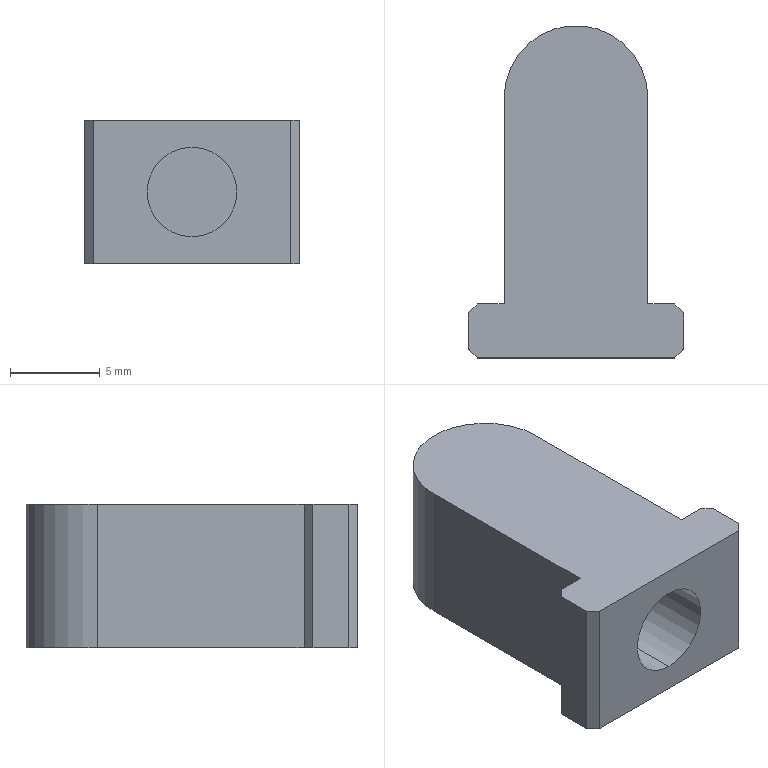Part | STEP file | limit pin-1 | 1 solid | 17 faces | box 12 x 18.5 x 8 mm | volume 1103 mm3 | plane 14 | cylinder 3 | commonest cylinder face diameters 5 x2 8 x1
STEP:
#1=CARTESIAN_POINT('',(0.,0.,0.));
#2=DIRECTION('',(0.,0.,1.));
#3=DIRECTION('',(1.,0.,0.));
#4=AXIS2_PLACEMENT_3D('',#1,#2,#3);
#5=CARTESIAN_POINT('',(0.,6.,1.5));
#6=VERTEX_POINT('',#5);
#7=CARTESIAN_POINT('',(0.,0.,1.5));
#8=VERTEX_POINT('',#7);
#9=CARTESIAN_POINT('',(0.,6.,1.5));
#10=DIRECTION('',(0.,-1.,0.));
#11=VECTOR('',#10,1.);
#12=LINE('',#9,#11);
#13=CARTESIAN_POINT('',(0.,6.,4.));
#14=DIRECTION('',(0.,-1.,0.));
#15=DIRECTION('',(0.,0.,-1.));
#16=AXIS2_PLACEMENT_3D('',#13,#14,#15);
#17=CYLINDRICAL_SURFACE('',#16,2.5);
#18=CARTESIAN_POINT('',(6.283,0.));
#19=DIRECTION('',(0.,1.));
#20=VECTOR('',#19,1.);
#21=LINE('',#18,#20);
#22=(GEOMETRIC_REPRESENTATION_CONTEXT(2)PARAMETRIC_REPRESENTATION_CONTEXT()REPRESENTATION_CONTEXT('',''));
#23=DEFINITIONAL_REPRESENTATION('',(#21),#22);
#24=PCURVE('',#17,#23);
#25=CARTESIAN_POINT('',(0.,6.,4.));
#26=DIRECTION('',(0.,-1.,0.));
#27=DIRECTION('',(0.,0.,-1.));
#28=AXIS2_PLACEMENT_3D('',#25,#26,#27);
#29=CYLINDRICAL_SURFACE('',#28,2.5);
#30=CARTESIAN_POINT('',(0.,0.));
#31=DIRECTION('',(0.,1.));
#32=VECTOR('',#31,1.);
#33=LINE('',#30,#32);
#34=(GEOMETRIC_REPRESENTATION_CONTEXT(2)PARAMETRIC_REPRESENTATION_CONTEXT()REPRESENTATION_CONTEXT('',''));
#35=DEFINITIONAL_REPRESENTATION('',(#33),#34);
#36=PCURVE('',#29,#35);
#37=SURFACE_CURVE('',#12,(#24,#36),.PCURVE_S1.);
#38=EDGE_CURVE('',#6,#8,#37,.T.);
#39=ORIENTED_EDGE('',*,*,#38,.T.);
#40=CARTESIAN_POINT('',(0.,0.,6.5));
#41=VERTEX_POINT('',#40);
#42=CARTESIAN_POINT('',(0.,0.,4.));
#43=DIRECTION('',(0.,-1.,0.));
#44=DIRECTION('',(0.,0.,-1.));
#45=AXIS2_PLACEMENT_3D('',#42,#43,#44);
#46=CIRCLE('',#45,2.5);
#47=CARTESIAN_POINT('',(0.,6.));
#48=DIRECTION('',(1.,0.));
#49=VECTOR('',#48,1.);
#50=LINE('',#47,#49);
#51=(GEOMETRIC_REPRESENTATION_CONTEXT(2)PARAMETRIC_REPRESENTATION_CONTEXT()REPRESENTATION_CONTEXT('',''));
#52=DEFINITIONAL_REPRESENTATION('',(#50),#51);
#53=PCURVE('',#17,#52);
#54=CARTESIAN_POINT('',(5.5,0.,8.));
#55=DIRECTION('',(0.,1.,0.));
#56=DIRECTION('',(0.,0.,1.));
#57=AXIS2_PLACEMENT_3D('',#54,#55,#56);
#58=PLANE('',#57);
#59=CARTESIAN_POINT('',(-6.5,-5.5));
#60=CARTESIAN_POINT('',(-6.5,-1.17));
#61=CARTESIAN_POINT('',(-2.75,-3.335));
#62=CARTESIAN_POINT('',(1.,-5.5));
#63=CARTESIAN_POINT('',(-2.75,-7.665));
#64=CARTESIAN_POINT('',(-6.5,-9.83));
#65=CARTESIAN_POINT('',(-6.5,-5.5));
#66=(BOUNDED_CURVE()B_SPLINE_CURVE(2,(#59,#60,#61,#62,#63,#64,#65),.UNSPECIFIED.,.T.,.F.)B_SPLINE_CURVE_WITH_KNOTS((1,2,2,2,2,1),(-2.094,0.,2.094,4.189,6.283,8.378),.UNSPECIFIED.)CURVE()GEOMETRIC_REPRESENTATION_ITEM()RATIONAL_B_SPLINE_CURVE((1.,0.5,1.,0.5,1.,0.5,1.))REPRESENTATION_ITEM(''));
#67=(GEOMETRIC_REPRESENTATION_CONTEXT(2)PARAMETRIC_REPRESENTATION_CONTEXT()REPRESENTATION_CONTEXT('',''));
#68=DEFINITIONAL_REPRESENTATION('',(#66),#67);
#69=PCURVE('',#58,#68);
#70=SURFACE_CURVE('',#46,(#53,#69),.PCURVE_S1.);
#71=EDGE_CURVE('',#41,#8,#70,.T.);
#72=ORIENTED_EDGE('',*,*,#71,.F.);
#73=CARTESIAN_POINT('',(0.,6.,6.5));
#74=VERTEX_POINT('',#73);
#75=CARTESIAN_POINT('',(0.,6.,6.5));
#76=DIRECTION('',(0.,-1.,0.));
#77=VECTOR('',#76,1.);
#78=LINE('',#75,#77);
#79=CARTESIAN_POINT('',(3.142,0.));
#80=DIRECTION('',(0.,1.));
#81=VECTOR('',#80,1.);
#82=LINE('',#79,#81);
#83=(GEOMETRIC_REPRESENTATION_CONTEXT(2)PARAMETRIC_REPRESENTATION_CONTEXT()REPRESENTATION_CONTEXT('',''));
#84=DEFINITIONAL_REPRESENTATION('',(#82),#83);
#85=PCURVE('',#17,#84);
#86=CARTESIAN_POINT('',(3.142,0.));
#87=DIRECTION('',(0.,1.));
#88=VECTOR('',#87,1.);
#89=LINE('',#86,#88);
#90=(GEOMETRIC_REPRESENTATION_CONTEXT(2)PARAMETRIC_REPRESENTATION_CONTEXT()REPRESENTATION_CONTEXT('',''));
#91=DEFINITIONAL_REPRESENTATION('',(#89),#90);
#92=PCURVE('',#29,#91);
#93=SURFACE_CURVE('',#78,(#85,#92),.PCURVE_S1.);
#94=EDGE_CURVE('',#74,#41,#93,.T.);
#95=ORIENTED_EDGE('',*,*,#94,.F.);
#96=CARTESIAN_POINT('',(0.,6.,4.));
#97=DIRECTION('',(0.,-1.,0.));
#98=DIRECTION('',(0.,0.,-1.));
#99=AXIS2_PLACEMENT_3D('',#96,#97,#98);
#100=CIRCLE('',#99,2.5);
#101=CARTESIAN_POINT('',(0.,0.));
#102=DIRECTION('',(1.,0.));
#103=VECTOR('',#102,1.);
#104=LINE('',#101,#103);
#105=(GEOMETRIC_REPRESENTATION_CONTEXT(2)PARAMETRIC_REPRESENTATION_CONTEXT()REPRESENTATION_CONTEXT('',''));
#106=DEFINITIONAL_REPRESENTATION('',(#104),#105);
#107=PCURVE('',#17,#106);
#108=CARTESIAN_POINT('',(0.,6.,4.));
#109=DIRECTION('',(0.,-1.,0.));
#110=DIRECTION('',(0.,0.,-1.));
#111=AXIS2_PLACEMENT_3D('',#108,#109,#110);
#112=PLANE('',#111);
#113=CARTESIAN_POINT('',(0.,0.));
#114=DIRECTION('',(1.,0.));
#115=AXIS2_PLACEMENT_2D('',#113,#114);
#116=CIRCLE('',#115,2.5);
#117=(GEOMETRIC_REPRESENTATION_CONTEXT(2)PARAMETRIC_REPRESENTATION_CONTEXT()REPRESENTATION_CONTEXT('',''));
#118=DEFINITIONAL_REPRESENTATION('',(#116),#117);
#119=PCURVE('',#112,#118);
#120=SURFACE_CURVE('',#100,(#107,#119),.PCURVE_S1.);
#121=EDGE_CURVE('',#74,#6,#120,.T.);
#122=ORIENTED_EDGE('',*,*,#121,.T.);
#123=EDGE_LOOP('',(#39,#72,#95,#122));
#124=FACE_BOUND('',#123,.F.);
#125=ADVANCED_FACE('',(#124),#17,.F.);
#126=CARTESIAN_POINT('',(5.5,0.,0.));
#127=VERTEX_POINT('',#126);
#128=CARTESIAN_POINT('',(6.,0.5,0.));
#129=VERTEX_POINT('',#128);
#130=CARTESIAN_POINT('',(5.5,0.,0.));
#131=DIRECTION('',(0.7071,0.7071,0.));
#132=VECTOR('',#131,1.);
#133=LINE('',#130,#132);
#134=CARTESIAN_POINT('',(5.5,0.,8.));
#135=DIRECTION('',(-0.7071,0.7071,0.));
#136=DIRECTION('',(-0.7071,-0.7071,0.));
#137=AXIS2_PLACEMENT_3D('',#134,#135,#136);
#138=PLANE('',#137);
#139=CARTESIAN_POINT('',(0.,-8.));
#140=DIRECTION('',(-1.,0.));
#141=VECTOR('',#140,1.);
#142=LINE('',#139,#141);
#143=(GEOMETRIC_REPRESENTATION_CONTEXT(2)PARAMETRIC_REPRESENTATION_CONTEXT()REPRESENTATION_CONTEXT('',''));
#144=DEFINITIONAL_REPRESENTATION('',(#142),#143);
#145=PCURVE('',#138,#144);
#146=CARTESIAN_POINT('',(0.,14.5,0.));
#147=DIRECTION('',(0.,0.,1.));
#148=DIRECTION('',(1.,0.,0.));
#149=AXIS2_PLACEMENT_3D('',#146,#147,#148);
#150=PLANE('',#149);
#151=CARTESIAN_POINT('',(5.5,-14.5));
#152=DIRECTION('',(0.7071,0.7071));
#153=VECTOR('',#152,1.);
#154=LINE('',#151,#153);
#155=(GEOMETRIC_REPRESENTATION_CONTEXT(2)PARAMETRIC_REPRESENTATION_CONTEXT()REPRESENTATION_CONTEXT('',''));
#156=DEFINITIONAL_REPRESENTATION('',(#154),#155);
#157=PCURVE('',#150,#156);
#158=SURFACE_CURVE('',#133,(#145,#157),.PCURVE_S1.);
#159=EDGE_CURVE('',#127,#129,#158,.T.);
#160=ORIENTED_EDGE('',*,*,#159,.T.);
#161=CARTESIAN_POINT('',(6.,0.5,8.));
#162=VERTEX_POINT('',#161);
#163=CARTESIAN_POINT('',(6.,0.5,8.));
#164=DIRECTION('',(0.,0.,-1.));
#165=VECTOR('',#164,1.);
#166=LINE('',#163,#165);
#167=CARTESIAN_POINT('',(-0.7071,0.));
#168=DIRECTION('',(0.,-1.));
#169=VECTOR('',#168,1.);
#170=LINE('',#167,#169);
#171=(GEOMETRIC_REPRESENTATION_CONTEXT(2)PARAMETRIC_REPRESENTATION_CONTEXT()REPRESENTATION_CONTEXT('',''));
#172=DEFINITIONAL_REPRESENTATION('',(#170),#171);
#173=PCURVE('',#138,#172);
#174=CARTESIAN_POINT('',(6.,0.5,8.));
#175=DIRECTION('',(-1.,0.,0.));
#176=DIRECTION('',(0.,0.,1.));
#177=AXIS2_PLACEMENT_3D('',#174,#175,#176);
#178=PLANE('',#177);
#179=CARTESIAN_POINT('',(0.,0.));
#180=DIRECTION('',(-1.,0.));
#181=VECTOR('',#180,1.);
#182=LINE('',#179,#181);
#183=(GEOMETRIC_REPRESENTATION_CONTEXT(2)PARAMETRIC_REPRESENTATION_CONTEXT()REPRESENTATION_CONTEXT('',''));
#184=DEFINITIONAL_REPRESENTATION('',(#182),#183);
#185=PCURVE('',#178,#184);
#186=SURFACE_CURVE('',#166,(#173,#185),.PCURVE_S1.);
#187=EDGE_CURVE('',#162,#129,#186,.T.);
#188=ORIENTED_EDGE('',*,*,#187,.F.);
#189=CARTESIAN_POINT('',(5.5,0.,8.));
#190=VERTEX_POINT('',#189);
#191=CARTESIAN_POINT('',(5.5,0.,8.));
#192=DIRECTION('',(0.7071,0.7071,0.));
#193=VECTOR('',#192,1.);
#194=LINE('',#191,#193);
#195=CARTESIAN_POINT('',(0.,0.));
#196=DIRECTION('',(-1.,0.));
#197=VECTOR('',#196,1.);
#198=LINE('',#195,#197);
#199=(GEOMETRIC_REPRESENTATION_CONTEXT(2)PARAMETRIC_REPRESENTATION_CONTEXT()REPRESENTATION_CONTEXT('',''));
#200=DEFINITIONAL_REPRESENTATION('',(#198),#199);
#201=PCURVE('',#138,#200);
#202=CARTESIAN_POINT('',(0.,14.5,8.));
#203=DIRECTION('',(0.,0.,1.));
#204=DIRECTION('',(1.,0.,0.));
#205=AXIS2_PLACEMENT_3D('',#202,#203,#204);
#206=PLANE('',#205);
#207=CARTESIAN_POINT('',(5.5,-14.5));
#208=DIRECTION('',(0.7071,0.7071));
#209=VECTOR('',#208,1.);
#210=LINE('',#207,#209);
#211=(GEOMETRIC_REPRESENTATION_CONTEXT(2)PARAMETRIC_REPRESENTATION_CONTEXT()REPRESENTATION_CONTEXT('',''));
#212=DEFINITIONAL_REPRESENTATION('',(#210),#211);
#213=PCURVE('',#206,#212);
#214=SURFACE_CURVE('',#194,(#201,#213),.PCURVE_S1.);
#215=EDGE_CURVE('',#190,#162,#214,.T.);
#216=ORIENTED_EDGE('',*,*,#215,.F.);
#217=CARTESIAN_POINT('',(5.5,0.,8.));
#218=DIRECTION('',(0.,0.,-1.));
#219=VECTOR('',#218,1.);
#220=LINE('',#217,#219);
#221=CARTESIAN_POINT('',(0.,0.));
#222=DIRECTION('',(0.,-1.));
#223=VECTOR('',#222,1.);
#224=LINE('',#221,#223);
#225=(GEOMETRIC_REPRESENTATION_CONTEXT(2)PARAMETRIC_REPRESENTATION_CONTEXT()REPRESENTATION_CONTEXT('',''));
#226=DEFINITIONAL_REPRESENTATION('',(#224),#225);
#227=PCURVE('',#138,#226);
#228=CARTESIAN_POINT('',(0.,0.));
#229=DIRECTION('',(-1.,0.));
#230=VECTOR('',#229,1.);
#231=LINE('',#228,#230);
#232=(GEOMETRIC_REPRESENTATION_CONTEXT(2)PARAMETRIC_REPRESENTATION_CONTEXT()REPRESENTATION_CONTEXT('',''));
#233=DEFINITIONAL_REPRESENTATION('',(#231),#232);
#234=PCURVE('',#58,#233);
#235=SURFACE_CURVE('',#220,(#227,#234),.PCURVE_S1.);
#236=EDGE_CURVE('',#190,#127,#235,.T.);
#237=ORIENTED_EDGE('',*,*,#236,.T.);
#238=EDGE_LOOP('',(#160,#188,#216,#237));
#239=FACE_BOUND('',#238,.T.);
#240=ADVANCED_FACE('',(#239),#138,.F.);
#241=CARTESIAN_POINT('',(6.,2.5,0.));
#242=VERTEX_POINT('',#241);
#243=CARTESIAN_POINT('',(6.,0.5,0.));
#244=DIRECTION('',(0.,1.,0.));
#245=VECTOR('',#244,1.);
#246=LINE('',#243,#245);
#247=CARTESIAN_POINT('',(-8.,0.));
#248=DIRECTION('',(0.,1.));
#249=VECTOR('',#248,1.);
#250=LINE('',#247,#249);
#251=(GEOMETRIC_REPRESENTATION_CONTEXT(2)PARAMETRIC_REPRESENTATION_CONTEXT()REPRESENTATION_CONTEXT('',''));
#252=DEFINITIONAL_REPRESENTATION('',(#250),#251);
#253=PCURVE('',#178,#252);
#254=CARTESIAN_POINT('',(6.,-14.));
#255=DIRECTION('',(0.,1.));
#256=VECTOR('',#255,1.);
#257=LINE('',#254,#256);
#258=(GEOMETRIC_REPRESENTATION_CONTEXT(2)PARAMETRIC_REPRESENTATION_CONTEXT()REPRESENTATION_CONTEXT('',''));
#259=DEFINITIONAL_REPRESENTATION('',(#257),#258);
#260=PCURVE('',#150,#259);
#261=SURFACE_CURVE('',#246,(#253,#260),.PCURVE_S1.);
#262=EDGE_CURVE('',#129,#242,#261,.T.);
#263=ORIENTED_EDGE('',*,*,#262,.T.);
#264=CARTESIAN_POINT('',(6.,2.5,8.));
#265=VERTEX_POINT('',#264);
#266=CARTESIAN_POINT('',(6.,2.5,8.));
#267=DIRECTION('',(0.,0.,-1.));
#268=VECTOR('',#267,1.);
#269=LINE('',#266,#268);
#270=CARTESIAN_POINT('',(0.,2.));
#271=DIRECTION('',(-1.,0.));
#272=VECTOR('',#271,1.);
#273=LINE('',#270,#272);
#274=(GEOMETRIC_REPRESENTATION_CONTEXT(2)PARAMETRIC_REPRESENTATION_CONTEXT()REPRESENTATION_CONTEXT('',''));
#275=DEFINITIONAL_REPRESENTATION('',(#273),#274);
#276=PCURVE('',#178,#275);
#277=CARTESIAN_POINT('',(6.,2.5,8.));
#278=DIRECTION('',(-0.7071,-0.7071,0.));
#279=DIRECTION('',(0.7071,-0.7071,0.));
#280=AXIS2_PLACEMENT_3D('',#277,#278,#279);
#281=PLANE('',#280);
#282=CARTESIAN_POINT('',(0.,0.));
#283=DIRECTION('',(0.,-1.));
#284=VECTOR('',#283,1.);
#285=LINE('',#282,#284);
#286=(GEOMETRIC_REPRESENTATION_CONTEXT(2)PARAMETRIC_REPRESENTATION_CONTEXT()REPRESENTATION_CONTEXT('',''));
#287=DEFINITIONAL_REPRESENTATION('',(#285),#286);
#288=PCURVE('',#281,#287);
#289=SURFACE_CURVE('',#269,(#276,#288),.PCURVE_S1.);
#290=EDGE_CURVE('',#265,#242,#289,.T.);
#291=ORIENTED_EDGE('',*,*,#290,.F.);
#292=CARTESIAN_POINT('',(6.,0.5,8.));
#293=DIRECTION('',(0.,1.,0.));
#294=VECTOR('',#293,1.);
#295=LINE('',#292,#294);
#296=CARTESIAN_POINT('',(0.,0.));
#297=DIRECTION('',(0.,1.));
#298=VECTOR('',#297,1.);
#299=LINE('',#296,#298);
#300=(GEOMETRIC_REPRESENTATION_CONTEXT(2)PARAMETRIC_REPRESENTATION_CONTEXT()REPRESENTATION_CONTEXT('',''));
#301=DEFINITIONAL_REPRESENTATION('',(#299),#300);
#302=PCURVE('',#178,#301);
#303=CARTESIAN_POINT('',(6.,-14.));
#304=DIRECTION('',(0.,1.));
#305=VECTOR('',#304,1.);
#306=LINE('',#303,#305);
#307=(GEOMETRIC_REPRESENTATION_CONTEXT(2)PARAMETRIC_REPRESENTATION_CONTEXT()REPRESENTATION_CONTEXT('',''));
#308=DEFINITIONAL_REPRESENTATION('',(#306),#307);
#309=PCURVE('',#206,#308);
#310=SURFACE_CURVE('',#295,(#302,#309),.PCURVE_S1.);
#311=EDGE_CURVE('',#162,#265,#310,.T.);
#312=ORIENTED_EDGE('',*,*,#311,.F.);
#313=ORIENTED_EDGE('',*,*,#187,.T.);
#314=EDGE_LOOP('',(#263,#291,#312,#313));
#315=FACE_BOUND('',#314,.T.);
#316=ADVANCED_FACE('',(#315),#178,.F.);
#317=CARTESIAN_POINT('',(5.5,3.,0.));
#318=VERTEX_POINT('',#317);
#319=CARTESIAN_POINT('',(6.,2.5,0.));
#320=DIRECTION('',(-0.7071,0.7071,0.));
#321=VECTOR('',#320,1.);
#322=LINE('',#319,#321);
#323=CARTESIAN_POINT('',(0.,-8.));
#324=DIRECTION('',(-1.,0.));
#325=VECTOR('',#324,1.);
#326=LINE('',#323,#325);
#327=(GEOMETRIC_REPRESENTATION_CONTEXT(2)PARAMETRIC_REPRESENTATION_CONTEXT()REPRESENTATION_CONTEXT('',''));
#328=DEFINITIONAL_REPRESENTATION('',(#326),#327);
#329=PCURVE('',#281,#328);
#330=CARTESIAN_POINT('',(6.,-12.));
#331=DIRECTION('',(-0.7071,0.7071));
#332=VECTOR('',#331,1.);
#333=LINE('',#330,#332);
#334=(GEOMETRIC_REPRESENTATION_CONTEXT(2)PARAMETRIC_REPRESENTATION_CONTEXT()REPRESENTATION_CONTEXT('',''));
#335=DEFINITIONAL_REPRESENTATION('',(#333),#334);
#336=PCURVE('',#150,#335);
#337=SURFACE_CURVE('',#322,(#329,#336),.PCURVE_S1.);
#338=EDGE_CURVE('',#242,#318,#337,.T.);
#339=ORIENTED_EDGE('',*,*,#338,.T.);
#340=CARTESIAN_POINT('',(5.5,3.,8.));
#341=VERTEX_POINT('',#340);
#342=CARTESIAN_POINT('',(5.5,3.,8.));
#343=DIRECTION('',(0.,0.,-1.));
#344=VECTOR('',#343,1.);
#345=LINE('',#342,#344);
#346=CARTESIAN_POINT('',(-0.7071,0.));
#347=DIRECTION('',(0.,-1.));
#348=VECTOR('',#347,1.);
#349=LINE('',#346,#348);
#350=(GEOMETRIC_REPRESENTATION_CONTEXT(2)PARAMETRIC_REPRESENTATION_CONTEXT()REPRESENTATION_CONTEXT('',''));
#351=DEFINITIONAL_REPRESENTATION('',(#349),#350);
#352=PCURVE('',#281,#351);
#353=CARTESIAN_POINT('',(5.5,3.,8.));
#354=DIRECTION('',(0.,-1.,0.));
#355=DIRECTION('',(0.,0.,-1.));
#356=AXIS2_PLACEMENT_3D('',#353,#354,#355);
#357=PLANE('',#356);
#358=CARTESIAN_POINT('',(0.,0.));
#359=DIRECTION('',(1.,0.));
#360=VECTOR('',#359,1.);
#361=LINE('',#358,#360);
#362=(GEOMETRIC_REPRESENTATION_CONTEXT(2)PARAMETRIC_REPRESENTATION_CONTEXT()REPRESENTATION_CONTEXT('',''));
#363=DEFINITIONAL_REPRESENTATION('',(#361),#362);
#364=PCURVE('',#357,#363);
#365=SURFACE_CURVE('',#345,(#352,#364),.PCURVE_S1.);
#366=EDGE_CURVE('',#341,#318,#365,.T.);
#367=ORIENTED_EDGE('',*,*,#366,.F.);
#368=CARTESIAN_POINT('',(6.,2.5,8.));
#369=DIRECTION('',(-0.7071,0.7071,0.));
#370=VECTOR('',#369,1.);
#371=LINE('',#368,#370);
#372=CARTESIAN_POINT('',(0.,0.));
#373=DIRECTION('',(-1.,0.));
#374=VECTOR('',#373,1.);
#375=LINE('',#372,#374);
#376=(GEOMETRIC_REPRESENTATION_CONTEXT(2)PARAMETRIC_REPRESENTATION_CONTEXT()REPRESENTATION_CONTEXT('',''));
#377=DEFINITIONAL_REPRESENTATION('',(#375),#376);
#378=PCURVE('',#281,#377);
#379=CARTESIAN_POINT('',(6.,-12.));
#380=DIRECTION('',(-0.7071,0.7071));
#381=VECTOR('',#380,1.);
#382=LINE('',#379,#381);
#383=(GEOMETRIC_REPRESENTATION_CONTEXT(2)PARAMETRIC_REPRESENTATION_CONTEXT()REPRESENTATION_CONTEXT('',''));
#384=DEFINITIONAL_REPRESENTATION('',(#382),#383);
#385=PCURVE('',#206,#384);
#386=SURFACE_CURVE('',#371,(#378,#385),.PCURVE_S1.);
#387=EDGE_CURVE('',#265,#341,#386,.T.);
#388=ORIENTED_EDGE('',*,*,#387,.F.);
#389=ORIENTED_EDGE('',*,*,#290,.T.);
#390=EDGE_LOOP('',(#339,#367,#388,#389));
#391=FACE_BOUND('',#390,.T.);
#392=ADVANCED_FACE('',(#391),#281,.F.);
#393=CARTESIAN_POINT('',(4.,3.,0.));
#394=VERTEX_POINT('',#393);
#395=CARTESIAN_POINT('',(5.5,3.,0.));
#396=DIRECTION('',(-1.,0.,0.));
#397=VECTOR('',#396,1.);
#398=LINE('',#395,#397);
#399=CARTESIAN_POINT('',(8.,0.));
#400=DIRECTION('',(0.,-1.));
#401=VECTOR('',#400,1.);
#402=LINE('',#399,#401);
#403=(GEOMETRIC_REPRESENTATION_CONTEXT(2)PARAMETRIC_REPRESENTATION_CONTEXT()REPRESENTATION_CONTEXT('',''));
#404=DEFINITIONAL_REPRESENTATION('',(#402),#403);
#405=PCURVE('',#357,#404);
#406=CARTESIAN_POINT('',(5.5,-11.5));
#407=DIRECTION('',(-1.,0.));
#408=VECTOR('',#407,1.);
#409=LINE('',#406,#408);
#410=(GEOMETRIC_REPRESENTATION_CONTEXT(2)PARAMETRIC_REPRESENTATION_CONTEXT()REPRESENTATION_CONTEXT('',''));
#411=DEFINITIONAL_REPRESENTATION('',(#409),#410);
#412=PCURVE('',#150,#411);
#413=SURFACE_CURVE('',#398,(#405,#412),.PCURVE_S1.);
#414=EDGE_CURVE('',#318,#394,#413,.T.);
#415=ORIENTED_EDGE('',*,*,#414,.T.);
#416=CARTESIAN_POINT('',(4.,3.,8.));
#417=VERTEX_POINT('',#416);
#418=CARTESIAN_POINT('',(4.,3.,8.));
#419=DIRECTION('',(0.,0.,-1.));
#420=VECTOR('',#419,1.);
#421=LINE('',#418,#420);
#422=CARTESIAN_POINT('',(0.,-1.5));
#423=DIRECTION('',(1.,0.));
#424=VECTOR('',#423,1.);
#425=LINE('',#422,#424);
#426=(GEOMETRIC_REPRESENTATION_CONTEXT(2)PARAMETRIC_REPRESENTATION_CONTEXT()REPRESENTATION_CONTEXT('',''));
#427=DEFINITIONAL_REPRESENTATION('',(#425),#426);
#428=PCURVE('',#357,#427);
#429=CARTESIAN_POINT('',(4.,3.,8.));
#430=DIRECTION('',(-1.,0.,0.));
#431=DIRECTION('',(0.,0.,1.));
#432=AXIS2_PLACEMENT_3D('',#429,#430,#431);
#433=PLANE('',#432);
#434=CARTESIAN_POINT('',(0.,0.));
#435=DIRECTION('',(-1.,0.));
#436=VECTOR('',#435,1.);
#437=LINE('',#434,#436);
#438=(GEOMETRIC_REPRESENTATION_CONTEXT(2)PARAMETRIC_REPRESENTATION_CONTEXT()REPRESENTATION_CONTEXT('',''));
#439=DEFINITIONAL_REPRESENTATION('',(#437),#438);
#440=PCURVE('',#433,#439);
#441=SURFACE_CURVE('',#421,(#428,#440),.PCURVE_S1.);
#442=EDGE_CURVE('',#417,#394,#441,.T.);
#443=ORIENTED_EDGE('',*,*,#442,.F.);
#444=CARTESIAN_POINT('',(5.5,3.,8.));
#445=DIRECTION('',(-1.,0.,0.));
#446=VECTOR('',#445,1.);
#447=LINE('',#444,#446);
#448=CARTESIAN_POINT('',(0.,0.));
#449=DIRECTION('',(0.,-1.));
#450=VECTOR('',#449,1.);
#451=LINE('',#448,#450);
#452=(GEOMETRIC_REPRESENTATION_CONTEXT(2)PARAMETRIC_REPRESENTATION_CONTEXT()REPRESENTATION_CONTEXT('',''));
#453=DEFINITIONAL_REPRESENTATION('',(#451),#452);
#454=PCURVE('',#357,#453);
#455=CARTESIAN_POINT('',(5.5,-11.5));
#456=DIRECTION('',(-1.,0.));
#457=VECTOR('',#456,1.);
#458=LINE('',#455,#457);
#459=(GEOMETRIC_REPRESENTATION_CONTEXT(2)PARAMETRIC_REPRESENTATION_CONTEXT()REPRESENTATION_CONTEXT('',''));
#460=DEFINITIONAL_REPRESENTATION('',(#458),#459);
#461=PCURVE('',#206,#460);
#462=SURFACE_CURVE('',#447,(#454,#461),.PCURVE_S1.);
#463=EDGE_CURVE('',#341,#417,#462,.T.);
#464=ORIENTED_EDGE('',*,*,#463,.F.);
#465=ORIENTED_EDGE('',*,*,#366,.T.);
#466=EDGE_LOOP('',(#415,#443,#464,#465));
#467=FACE_BOUND('',#466,.T.);
#468=ADVANCED_FACE('',(#467),#357,.F.);
#469=CARTESIAN_POINT('',(4.,14.5,0.));
#470=VERTEX_POINT('',#469);
#471=CARTESIAN_POINT('',(4.,3.,0.));
#472=DIRECTION('',(0.,1.,0.));
#473=VECTOR('',#472,1.);
#474=LINE('',#471,#473);
#475=CARTESIAN_POINT('',(-8.,0.));
#476=DIRECTION('',(0.,1.));
#477=VECTOR('',#476,1.);
#478=LINE('',#475,#477);
#479=(GEOMETRIC_REPRESENTATION_CONTEXT(2)PARAMETRIC_REPRESENTATION_CONTEXT()REPRESENTATION_CONTEXT('',''));
#480=DEFINITIONAL_REPRESENTATION('',(#478),#479);
#481=PCURVE('',#433,#480);
#482=CARTESIAN_POINT('',(4.,-11.5));
#483=DIRECTION('',(0.,1.));
#484=VECTOR('',#483,1.);
#485=LINE('',#482,#484);
#486=(GEOMETRIC_REPRESENTATION_CONTEXT(2)PARAMETRIC_REPRESENTATION_CONTEXT()REPRESENTATION_CONTEXT('',''));
#487=DEFINITIONAL_REPRESENTATION('',(#485),#486);
#488=PCURVE('',#150,#487);
#489=SURFACE_CURVE('',#474,(#481,#488),.PCURVE_S1.);
#490=EDGE_CURVE('',#394,#470,#489,.T.);
#491=ORIENTED_EDGE('',*,*,#490,.T.);
#492=CARTESIAN_POINT('',(4.,14.5,8.));
#493=VERTEX_POINT('',#492);
#494=CARTESIAN_POINT('',(4.,14.5,8.));
#495=DIRECTION('',(0.,0.,-1.));
#496=VECTOR('',#495,1.);
#497=LINE('',#494,#496);
#498=CARTESIAN_POINT('',(0.,11.5));
#499=DIRECTION('',(-1.,0.));
#500=VECTOR('',#499,1.);
#501=LINE('',#498,#500);
#502=(GEOMETRIC_REPRESENTATION_CONTEXT(2)PARAMETRIC_REPRESENTATION_CONTEXT()REPRESENTATION_CONTEXT('',''));
#503=DEFINITIONAL_REPRESENTATION('',(#501),#502);
#504=PCURVE('',#433,#503);
#505=CARTESIAN_POINT('',(0.,14.5,8.));
#506=DIRECTION('',(0.,0.,-1.));
#507=DIRECTION('',(-1.,0.,0.));
#508=AXIS2_PLACEMENT_3D('',#505,#506,#507);
#509=CYLINDRICAL_SURFACE('',#508,4.);
#510=CARTESIAN_POINT('',(3.142,0.));
#511=DIRECTION('',(0.,1.));
#512=VECTOR('',#511,1.);
#513=LINE('',#510,#512);
#514=(GEOMETRIC_REPRESENTATION_CONTEXT(2)PARAMETRIC_REPRESENTATION_CONTEXT()REPRESENTATION_CONTEXT('',''));
#515=DEFINITIONAL_REPRESENTATION('',(#513),#514);
#516=PCURVE('',#509,#515);
#517=SURFACE_CURVE('',#497,(#504,#516),.PCURVE_S1.);
#518=EDGE_CURVE('',#493,#470,#517,.T.);
#519=ORIENTED_EDGE('',*,*,#518,.F.);
#520=CARTESIAN_POINT('',(4.,3.,8.));
#521=DIRECTION('',(0.,1.,0.));
#522=VECTOR('',#521,1.);
#523=LINE('',#520,#522);
#524=CARTESIAN_POINT('',(0.,0.));
#525=DIRECTION('',(0.,1.));
#526=VECTOR('',#525,1.);
#527=LINE('',#524,#526);
#528=(GEOMETRIC_REPRESENTATION_CONTEXT(2)PARAMETRIC_REPRESENTATION_CONTEXT()REPRESENTATION_CONTEXT('',''));
#529=DEFINITIONAL_REPRESENTATION('',(#527),#528);
#530=PCURVE('',#433,#529);
#531=CARTESIAN_POINT('',(4.,-11.5));
#532=DIRECTION('',(0.,1.));
#533=VECTOR('',#532,1.);
#534=LINE('',#531,#533);
#535=(GEOMETRIC_REPRESENTATION_CONTEXT(2)PARAMETRIC_REPRESENTATION_CONTEXT()REPRESENTATION_CONTEXT('',''));
#536=DEFINITIONAL_REPRESENTATION('',(#534),#535);
#537=PCURVE('',#206,#536);
#538=SURFACE_CURVE('',#523,(#530,#537),.PCURVE_S1.);
#539=EDGE_CURVE('',#417,#493,#538,.T.);
#540=ORIENTED_EDGE('',*,*,#539,.F.);
#541=ORIENTED_EDGE('',*,*,#442,.T.);
#542=EDGE_LOOP('',(#491,#519,#540,#541));
#543=FACE_BOUND('',#542,.T.);
#544=ADVANCED_FACE('',(#543),#433,.F.);
#545=CARTESIAN_POINT('',(-4.,14.5,0.));
#546=VERTEX_POINT('',#545);
#547=CARTESIAN_POINT('',(0.,14.5,0.));
#548=DIRECTION('',(0.,0.,1.));
#549=DIRECTION('',(1.,0.,0.));
#550=AXIS2_PLACEMENT_3D('',#547,#548,#549);
#551=CIRCLE('',#550,4.);
#552=CARTESIAN_POINT('',(3.142,8.));
#553=DIRECTION('',(-1.,0.));
#554=VECTOR('',#553,1.);
#555=LINE('',#552,#554);
#556=(GEOMETRIC_REPRESENTATION_CONTEXT(2)PARAMETRIC_REPRESENTATION_CONTEXT()REPRESENTATION_CONTEXT('',''));
#557=DEFINITIONAL_REPRESENTATION('',(#555),#556);
#558=PCURVE('',#509,#557);
#559=CARTESIAN_POINT('',(0.,0.));
#560=DIRECTION('',(1.,0.));
#561=AXIS2_PLACEMENT_2D('',#559,#560);
#562=CIRCLE('',#561,4.);
#563=(GEOMETRIC_REPRESENTATION_CONTEXT(2)PARAMETRIC_REPRESENTATION_CONTEXT()REPRESENTATION_CONTEXT('',''));
#564=DEFINITIONAL_REPRESENTATION('',(#562),#563);
#565=PCURVE('',#150,#564);
#566=SURFACE_CURVE('',#551,(#558,#565),.PCURVE_S1.);
#567=EDGE_CURVE('',#470,#546,#566,.T.);
#568=ORIENTED_EDGE('',*,*,#567,.T.);
#569=CARTESIAN_POINT('',(-4.,14.5,8.));
#570=VERTEX_POINT('',#569);
#571=CARTESIAN_POINT('',(-4.,14.5,8.));
#572=DIRECTION('',(0.,0.,-1.));
#573=VECTOR('',#572,1.);
#574=LINE('',#571,#573);
#575=CARTESIAN_POINT('',(0.,0.));
#576=DIRECTION('',(0.,1.));
#577=VECTOR('',#576,1.);
#578=LINE('',#575,#577);
#579=(GEOMETRIC_REPRESENTATION_CONTEXT(2)PARAMETRIC_REPRESENTATION_CONTEXT()REPRESENTATION_CONTEXT('',''));
#580=DEFINITIONAL_REPRESENTATION('',(#578),#579);
#581=PCURVE('',#509,#580);
#582=CARTESIAN_POINT('',(-4.,3.,8.));
#583=DIRECTION('',(1.,0.,0.));
#584=DIRECTION('',(0.,0.,-1.));
#585=AXIS2_PLACEMENT_3D('',#582,#583,#584);
#586=PLANE('',#585);
#587=CARTESIAN_POINT('',(0.,11.5));
#588=DIRECTION('',(1.,0.));
#589=VECTOR('',#588,1.);
#590=LINE('',#587,#589);
#591=(GEOMETRIC_REPRESENTATION_CONTEXT(2)PARAMETRIC_REPRESENTATION_CONTEXT()REPRESENTATION_CONTEXT('',''));
#592=DEFINITIONAL_REPRESENTATION('',(#590),#591);
#593=PCURVE('',#586,#592);
#594=SURFACE_CURVE('',#574,(#581,#593),.PCURVE_S1.);
#595=EDGE_CURVE('',#570,#546,#594,.T.);
#596=ORIENTED_EDGE('',*,*,#595,.F.);
#597=CARTESIAN_POINT('',(0.,14.5,8.));
#598=DIRECTION('',(0.,0.,1.));
#599=DIRECTION('',(1.,0.,0.));
#600=AXIS2_PLACEMENT_3D('',#597,#598,#599);
#601=CIRCLE('',#600,4.);
#602=CARTESIAN_POINT('',(3.142,0.));
#603=DIRECTION('',(-1.,0.));
#604=VECTOR('',#603,1.);
#605=LINE('',#602,#604);
#606=(GEOMETRIC_REPRESENTATION_CONTEXT(2)PARAMETRIC_REPRESENTATION_CONTEXT()REPRESENTATION_CONTEXT('',''));
#607=DEFINITIONAL_REPRESENTATION('',(#605),#606);
#608=PCURVE('',#509,#607);
#609=CARTESIAN_POINT('',(0.,0.));
#610=DIRECTION('',(1.,0.));
#611=AXIS2_PLACEMENT_2D('',#609,#610);
#612=CIRCLE('',#611,4.);
#613=(GEOMETRIC_REPRESENTATION_CONTEXT(2)PARAMETRIC_REPRESENTATION_CONTEXT()REPRESENTATION_CONTEXT('',''));
#614=DEFINITIONAL_REPRESENTATION('',(#612),#613);
#615=PCURVE('',#206,#614);
#616=SURFACE_CURVE('',#601,(#608,#615),.PCURVE_S1.);
#617=EDGE_CURVE('',#493,#570,#616,.T.);
#618=ORIENTED_EDGE('',*,*,#617,.F.);
#619=ORIENTED_EDGE('',*,*,#518,.T.);
#620=EDGE_LOOP('',(#568,#596,#618,#619));
#621=FACE_BOUND('',#620,.T.);
#622=ADVANCED_FACE('',(#621),#509,.T.);
#623=CARTESIAN_POINT('',(-4.,3.,0.));
#624=VERTEX_POINT('',#623);
#625=CARTESIAN_POINT('',(-4.,3.,0.));
#626=DIRECTION('',(0.,-1.,0.));
#627=VECTOR('',#626,1.);
#628=LINE('',#625,#627);
#629=CARTESIAN_POINT('',(8.,0.));
#630=DIRECTION('',(0.,-1.));
#631=VECTOR('',#630,1.);
#632=LINE('',#629,#631);
#633=(GEOMETRIC_REPRESENTATION_CONTEXT(2)PARAMETRIC_REPRESENTATION_CONTEXT()REPRESENTATION_CONTEXT('',''));
#634=DEFINITIONAL_REPRESENTATION('',(#632),#633);
#635=PCURVE('',#586,#634);
#636=CARTESIAN_POINT('',(-4.,-11.5));
#637=DIRECTION('',(0.,-1.));
#638=VECTOR('',#637,1.);
#639=LINE('',#636,#638);
#640=(GEOMETRIC_REPRESENTATION_CONTEXT(2)PARAMETRIC_REPRESENTATION_CONTEXT()REPRESENTATION_CONTEXT('',''));
#641=DEFINITIONAL_REPRESENTATION('',(#639),#640);
#642=PCURVE('',#150,#641);
#643=SURFACE_CURVE('',#628,(#635,#642),.PCURVE_S1.);
#644=EDGE_CURVE('',#546,#624,#643,.T.);
#645=ORIENTED_EDGE('',*,*,#644,.T.);
#646=CARTESIAN_POINT('',(-4.,3.,8.));
#647=VERTEX_POINT('',#646);
#648=CARTESIAN_POINT('',(-4.,3.,8.));
#649=DIRECTION('',(0.,0.,-1.));
#650=VECTOR('',#649,1.);
#651=LINE('',#648,#650);
#652=CARTESIAN_POINT('',(0.,0.));
#653=DIRECTION('',(1.,0.));
#654=VECTOR('',#653,1.);
#655=LINE('',#652,#654);
#656=(GEOMETRIC_REPRESENTATION_CONTEXT(2)PARAMETRIC_REPRESENTATION_CONTEXT()REPRESENTATION_CONTEXT('',''));
#657=DEFINITIONAL_REPRESENTATION('',(#655),#656);
#658=PCURVE('',#586,#657);
#659=CARTESIAN_POINT('',(-4.,3.,8.));
#660=DIRECTION('',(0.,-1.,0.));
#661=DIRECTION('',(0.,0.,-1.));
#662=AXIS2_PLACEMENT_3D('',#659,#660,#661);
#663=PLANE('',#662);
#664=CARTESIAN_POINT('',(0.,0.));
#665=DIRECTION('',(1.,0.));
#666=VECTOR('',#665,1.);
#667=LINE('',#664,#666);
#668=(GEOMETRIC_REPRESENTATION_CONTEXT(2)PARAMETRIC_REPRESENTATION_CONTEXT()REPRESENTATION_CONTEXT('',''));
#669=DEFINITIONAL_REPRESENTATION('',(#667),#668);
#670=PCURVE('',#663,#669);
#671=SURFACE_CURVE('',#651,(#658,#670),.PCURVE_S1.);
#672=EDGE_CURVE('',#647,#624,#671,.T.);
#673=ORIENTED_EDGE('',*,*,#672,.F.);
#674=CARTESIAN_POINT('',(-4.,3.,8.));
#675=DIRECTION('',(0.,-1.,0.));
#676=VECTOR('',#675,1.);
#677=LINE('',#674,#676);
#678=CARTESIAN_POINT('',(0.,0.));
#679=DIRECTION('',(0.,-1.));
#680=VECTOR('',#679,1.);
#681=LINE('',#678,#680);
#682=(GEOMETRIC_REPRESENTATION_CONTEXT(2)PARAMETRIC_REPRESENTATION_CONTEXT()REPRESENTATION_CONTEXT('',''));
#683=DEFINITIONAL_REPRESENTATION('',(#681),#682);
#684=PCURVE('',#586,#683);
#685=CARTESIAN_POINT('',(-4.,-11.5));
#686=DIRECTION('',(0.,-1.));
#687=VECTOR('',#686,1.);
#688=LINE('',#685,#687);
#689=(GEOMETRIC_REPRESENTATION_CONTEXT(2)PARAMETRIC_REPRESENTATION_CONTEXT()REPRESENTATION_CONTEXT('',''));
#690=DEFINITIONAL_REPRESENTATION('',(#688),#689);
#691=PCURVE('',#206,#690);
#692=SURFACE_CURVE('',#677,(#684,#691),.PCURVE_S1.);
#693=EDGE_CURVE('',#570,#647,#692,.T.);
#694=ORIENTED_EDGE('',*,*,#693,.F.);
#695=ORIENTED_EDGE('',*,*,#595,.T.);
#696=EDGE_LOOP('',(#645,#673,#694,#695));
#697=FACE_BOUND('',#696,.T.);
#698=ADVANCED_FACE('',(#697),#586,.F.);
#699=CARTESIAN_POINT('',(-5.5,3.,0.));
#700=VERTEX_POINT('',#699);
#701=CARTESIAN_POINT('',(-4.,3.,0.));
#702=DIRECTION('',(-1.,0.,0.));
#703=VECTOR('',#702,1.);
#704=LINE('',#701,#703);
#705=CARTESIAN_POINT('',(8.,0.));
#706=DIRECTION('',(0.,-1.));
#707=VECTOR('',#706,1.);
#708=LINE('',#705,#707);
#709=(GEOMETRIC_REPRESENTATION_CONTEXT(2)PARAMETRIC_REPRESENTATION_CONTEXT()REPRESENTATION_CONTEXT('',''));
#710=DEFINITIONAL_REPRESENTATION('',(#708),#709);
#711=PCURVE('',#663,#710);
#712=CARTESIAN_POINT('',(-4.,-11.5));
#713=DIRECTION('',(-1.,0.));
#714=VECTOR('',#713,1.);
#715=LINE('',#712,#714);
#716=(GEOMETRIC_REPRESENTATION_CONTEXT(2)PARAMETRIC_REPRESENTATION_CONTEXT()REPRESENTATION_CONTEXT('',''));
#717=DEFINITIONAL_REPRESENTATION('',(#715),#716);
#718=PCURVE('',#150,#717);
#719=SURFACE_CURVE('',#704,(#711,#718),.PCURVE_S1.);
#720=EDGE_CURVE('',#624,#700,#719,.T.);
#721=ORIENTED_EDGE('',*,*,#720,.T.);
#722=CARTESIAN_POINT('',(-5.5,3.,8.));
#723=VERTEX_POINT('',#722);
#724=CARTESIAN_POINT('',(-5.5,3.,8.));
#725=DIRECTION('',(0.,0.,-1.));
#726=VECTOR('',#725,1.);
#727=LINE('',#724,#726);
#728=CARTESIAN_POINT('',(0.,-1.5));
#729=DIRECTION('',(1.,0.));
#730=VECTOR('',#729,1.);
#731=LINE('',#728,#730);
#732=(GEOMETRIC_REPRESENTATION_CONTEXT(2)PARAMETRIC_REPRESENTATION_CONTEXT()REPRESENTATION_CONTEXT('',''));
#733=DEFINITIONAL_REPRESENTATION('',(#731),#732);
#734=PCURVE('',#663,#733);
#735=CARTESIAN_POINT('',(-5.5,3.,8.));
#736=DIRECTION('',(0.7071,-0.7071,0.));
#737=DIRECTION('',(0.7071,0.7071,0.));
#738=AXIS2_PLACEMENT_3D('',#735,#736,#737);
#739=PLANE('',#738);
#740=CARTESIAN_POINT('',(0.,0.));
#741=DIRECTION('',(0.,-1.));
#742=VECTOR('',#741,1.);
#743=LINE('',#740,#742);
#744=(GEOMETRIC_REPRESENTATION_CONTEXT(2)PARAMETRIC_REPRESENTATION_CONTEXT()REPRESENTATION_CONTEXT('',''));
#745=DEFINITIONAL_REPRESENTATION('',(#743),#744);
#746=PCURVE('',#739,#745);
#747=SURFACE_CURVE('',#727,(#734,#746),.PCURVE_S1.);
#748=EDGE_CURVE('',#723,#700,#747,.T.);
#749=ORIENTED_EDGE('',*,*,#748,.F.);
#750=CARTESIAN_POINT('',(-4.,3.,8.));
#751=DIRECTION('',(-1.,0.,0.));
#752=VECTOR('',#751,1.);
#753=LINE('',#750,#752);
#754=CARTESIAN_POINT('',(0.,0.));
#755=DIRECTION('',(0.,-1.));
#756=VECTOR('',#755,1.);
#757=LINE('',#754,#756);
#758=(GEOMETRIC_REPRESENTATION_CONTEXT(2)PARAMETRIC_REPRESENTATION_CONTEXT()REPRESENTATION_CONTEXT('',''));
#759=DEFINITIONAL_REPRESENTATION('',(#757),#758);
#760=PCURVE('',#663,#759);
#761=CARTESIAN_POINT('',(-4.,-11.5));
#762=DIRECTION('',(-1.,0.));
#763=VECTOR('',#762,1.);
#764=LINE('',#761,#763);
#765=(GEOMETRIC_REPRESENTATION_CONTEXT(2)PARAMETRIC_REPRESENTATION_CONTEXT()REPRESENTATION_CONTEXT('',''));
#766=DEFINITIONAL_REPRESENTATION('',(#764),#765);
#767=PCURVE('',#206,#766);
#768=SURFACE_CURVE('',#753,(#760,#767),.PCURVE_S1.);
#769=EDGE_CURVE('',#647,#723,#768,.T.);
#770=ORIENTED_EDGE('',*,*,#769,.F.);
#771=ORIENTED_EDGE('',*,*,#672,.T.);
#772=EDGE_LOOP('',(#721,#749,#770,#771));
#773=FACE_BOUND('',#772,.T.);
#774=ADVANCED_FACE('',(#773),#663,.F.);
#775=CARTESIAN_POINT('',(-6.,2.5,0.));
#776=VERTEX_POINT('',#775);
#777=CARTESIAN_POINT('',(-5.5,3.,0.));
#778=DIRECTION('',(-0.7071,-0.7071,0.));
#779=VECTOR('',#778,1.);
#780=LINE('',#777,#779);
#781=CARTESIAN_POINT('',(0.,-8.));
#782=DIRECTION('',(-1.,0.));
#783=VECTOR('',#782,1.);
#784=LINE('',#781,#783);
#785=(GEOMETRIC_REPRESENTATION_CONTEXT(2)PARAMETRIC_REPRESENTATION_CONTEXT()REPRESENTATION_CONTEXT('',''));
#786=DEFINITIONAL_REPRESENTATION('',(#784),#785);
#787=PCURVE('',#739,#786);
#788=CARTESIAN_POINT('',(-5.5,-11.5));
#789=DIRECTION('',(-0.7071,-0.7071));
#790=VECTOR('',#789,1.);
#791=LINE('',#788,#790);
#792=(GEOMETRIC_REPRESENTATION_CONTEXT(2)PARAMETRIC_REPRESENTATION_CONTEXT()REPRESENTATION_CONTEXT('',''));
#793=DEFINITIONAL_REPRESENTATION('',(#791),#792);
#794=PCURVE('',#150,#793);
#795=SURFACE_CURVE('',#780,(#787,#794),.PCURVE_S1.);
#796=EDGE_CURVE('',#700,#776,#795,.T.);
#797=ORIENTED_EDGE('',*,*,#796,.T.);
#798=CARTESIAN_POINT('',(-6.,2.5,8.));
#799=VERTEX_POINT('',#798);
#800=CARTESIAN_POINT('',(-6.,2.5,8.));
#801=DIRECTION('',(0.,0.,-1.));
#802=VECTOR('',#801,1.);
#803=LINE('',#800,#802);
#804=CARTESIAN_POINT('',(-0.7071,0.));
#805=DIRECTION('',(0.,-1.));
#806=VECTOR('',#805,1.);
#807=LINE('',#804,#806);
#808=(GEOMETRIC_REPRESENTATION_CONTEXT(2)PARAMETRIC_REPRESENTATION_CONTEXT()REPRESENTATION_CONTEXT('',''));
#809=DEFINITIONAL_REPRESENTATION('',(#807),#808);
#810=PCURVE('',#739,#809);
#811=CARTESIAN_POINT('',(-6.,2.5,8.));
#812=DIRECTION('',(1.,0.,0.));
#813=DIRECTION('',(0.,0.,-1.));
#814=AXIS2_PLACEMENT_3D('',#811,#812,#813);
#815=PLANE('',#814);
#816=CARTESIAN_POINT('',(0.,0.));
#817=DIRECTION('',(1.,0.));
#818=VECTOR('',#817,1.);
#819=LINE('',#816,#818);
#820=(GEOMETRIC_REPRESENTATION_CONTEXT(2)PARAMETRIC_REPRESENTATION_CONTEXT()REPRESENTATION_CONTEXT('',''));
#821=DEFINITIONAL_REPRESENTATION('',(#819),#820);
#822=PCURVE('',#815,#821);
#823=SURFACE_CURVE('',#803,(#810,#822),.PCURVE_S1.);
#824=EDGE_CURVE('',#799,#776,#823,.T.);
#825=ORIENTED_EDGE('',*,*,#824,.F.);
#826=CARTESIAN_POINT('',(-5.5,3.,8.));
#827=DIRECTION('',(-0.7071,-0.7071,0.));
#828=VECTOR('',#827,1.);
#829=LINE('',#826,#828);
#830=CARTESIAN_POINT('',(0.,0.));
#831=DIRECTION('',(-1.,0.));
#832=VECTOR('',#831,1.);
#833=LINE('',#830,#832);
#834=(GEOMETRIC_REPRESENTATION_CONTEXT(2)PARAMETRIC_REPRESENTATION_CONTEXT()REPRESENTATION_CONTEXT('',''));
#835=DEFINITIONAL_REPRESENTATION('',(#833),#834);
#836=PCURVE('',#739,#835);
#837=CARTESIAN_POINT('',(-5.5,-11.5));
#838=DIRECTION('',(-0.7071,-0.7071));
#839=VECTOR('',#838,1.);
#840=LINE('',#837,#839);
#841=(GEOMETRIC_REPRESENTATION_CONTEXT(2)PARAMETRIC_REPRESENTATION_CONTEXT()REPRESENTATION_CONTEXT('',''));
#842=DEFINITIONAL_REPRESENTATION('',(#840),#841);
#843=PCURVE('',#206,#842);
#844=SURFACE_CURVE('',#829,(#836,#843),.PCURVE_S1.);
#845=EDGE_CURVE('',#723,#799,#844,.T.);
#846=ORIENTED_EDGE('',*,*,#845,.F.);
#847=ORIENTED_EDGE('',*,*,#748,.T.);
#848=EDGE_LOOP('',(#797,#825,#846,#847));
#849=FACE_BOUND('',#848,.T.);
#850=ADVANCED_FACE('',(#849),#739,.F.);
#851=CARTESIAN_POINT('',(-6.,0.5,0.));
#852=VERTEX_POINT('',#851);
#853=CARTESIAN_POINT('',(-6.,2.5,0.));
#854=DIRECTION('',(0.,-1.,0.));
#855=VECTOR('',#854,1.);
#856=LINE('',#853,#855);
#857=CARTESIAN_POINT('',(8.,0.));
#858=DIRECTION('',(0.,-1.));
#859=VECTOR('',#858,1.);
#860=LINE('',#857,#859);
#861=(GEOMETRIC_REPRESENTATION_CONTEXT(2)PARAMETRIC_REPRESENTATION_CONTEXT()REPRESENTATION_CONTEXT('',''));
#862=DEFINITIONAL_REPRESENTATION('',(#860),#861);
#863=PCURVE('',#815,#862);
#864=CARTESIAN_POINT('',(-6.,-12.));
#865=DIRECTION('',(0.,-1.));
#866=VECTOR('',#865,1.);
#867=LINE('',#864,#866);
#868=(GEOMETRIC_REPRESENTATION_CONTEXT(2)PARAMETRIC_REPRESENTATION_CONTEXT()REPRESENTATION_CONTEXT('',''));
#869=DEFINITIONAL_REPRESENTATION('',(#867),#868);
#870=PCURVE('',#150,#869);
#871=SURFACE_CURVE('',#856,(#863,#870),.PCURVE_S1.);
#872=EDGE_CURVE('',#776,#852,#871,.T.);
#873=ORIENTED_EDGE('',*,*,#872,.T.);
#874=CARTESIAN_POINT('',(-6.,0.5,8.));
#875=VERTEX_POINT('',#874);
#876=CARTESIAN_POINT('',(-6.,0.5,8.));
#877=DIRECTION('',(0.,0.,-1.));
#878=VECTOR('',#877,1.);
#879=LINE('',#876,#878);
#880=CARTESIAN_POINT('',(0.,-2.));
#881=DIRECTION('',(1.,0.));
#882=VECTOR('',#881,1.);
#883=LINE('',#880,#882);
#884=(GEOMETRIC_REPRESENTATION_CONTEXT(2)PARAMETRIC_REPRESENTATION_CONTEXT()REPRESENTATION_CONTEXT('',''));
#885=DEFINITIONAL_REPRESENTATION('',(#883),#884);
#886=PCURVE('',#815,#885);
#887=CARTESIAN_POINT('',(-5.5,0.,8.));
#888=DIRECTION('',(0.7071,0.7071,0.));
#889=DIRECTION('',(-0.7071,0.7071,0.));
#890=AXIS2_PLACEMENT_3D('',#887,#888,#889);
#891=PLANE('',#890);
#892=CARTESIAN_POINT('',(0.7071,0.));
#893=DIRECTION('',(0.,-1.));
#894=VECTOR('',#893,1.);
#895=LINE('',#892,#894);
#896=(GEOMETRIC_REPRESENTATION_CONTEXT(2)PARAMETRIC_REPRESENTATION_CONTEXT()REPRESENTATION_CONTEXT('',''));
#897=DEFINITIONAL_REPRESENTATION('',(#895),#896);
#898=PCURVE('',#891,#897);
#899=SURFACE_CURVE('',#879,(#886,#898),.PCURVE_S1.);
#900=EDGE_CURVE('',#875,#852,#899,.T.);
#901=ORIENTED_EDGE('',*,*,#900,.F.);
#902=CARTESIAN_POINT('',(-6.,2.5,8.));
#903=DIRECTION('',(0.,-1.,0.));
#904=VECTOR('',#903,1.);
#905=LINE('',#902,#904);
#906=CARTESIAN_POINT('',(0.,0.));
#907=DIRECTION('',(0.,-1.));
#908=VECTOR('',#907,1.);
#909=LINE('',#906,#908);
#910=(GEOMETRIC_REPRESENTATION_CONTEXT(2)PARAMETRIC_REPRESENTATION_CONTEXT()REPRESENTATION_CONTEXT('',''));
#911=DEFINITIONAL_REPRESENTATION('',(#909),#910);
#912=PCURVE('',#815,#911);
#913=CARTESIAN_POINT('',(-6.,-12.));
#914=DIRECTION('',(0.,-1.));
#915=VECTOR('',#914,1.);
#916=LINE('',#913,#915);
#917=(GEOMETRIC_REPRESENTATION_CONTEXT(2)PARAMETRIC_REPRESENTATION_CONTEXT()REPRESENTATION_CONTEXT('',''));
#918=DEFINITIONAL_REPRESENTATION('',(#916),#917);
#919=PCURVE('',#206,#918);
#920=SURFACE_CURVE('',#905,(#912,#919),.PCURVE_S1.);
#921=EDGE_CURVE('',#799,#875,#920,.T.);
#922=ORIENTED_EDGE('',*,*,#921,.F.);
#923=ORIENTED_EDGE('',*,*,#824,.T.);
#924=EDGE_LOOP('',(#873,#901,#922,#923));
#925=FACE_BOUND('',#924,.T.);
#926=ADVANCED_FACE('',(#925),#815,.F.);
#927=CARTESIAN_POINT('',(-5.5,0.,0.));
#928=VERTEX_POINT('',#927);
#929=CARTESIAN_POINT('',(-5.5,0.,0.));
#930=DIRECTION('',(0.7071,-0.7071,0.));
#931=VECTOR('',#930,1.);
#932=LINE('',#929,#931);
#933=CARTESIAN_POINT('',(0.,-8.));
#934=DIRECTION('',(-1.,0.));
#935=VECTOR('',#934,1.);
#936=LINE('',#933,#935);
#937=(GEOMETRIC_REPRESENTATION_CONTEXT(2)PARAMETRIC_REPRESENTATION_CONTEXT()REPRESENTATION_CONTEXT('',''));
#938=DEFINITIONAL_REPRESENTATION('',(#936),#937);
#939=PCURVE('',#891,#938);
#940=CARTESIAN_POINT('',(-5.5,-14.5));
#941=DIRECTION('',(0.7071,-0.7071));
#942=VECTOR('',#941,1.);
#943=LINE('',#940,#942);
#944=(GEOMETRIC_REPRESENTATION_CONTEXT(2)PARAMETRIC_REPRESENTATION_CONTEXT()REPRESENTATION_CONTEXT('',''));
#945=DEFINITIONAL_REPRESENTATION('',(#943),#944);
#946=PCURVE('',#150,#945);
#947=SURFACE_CURVE('',#932,(#939,#946),.PCURVE_S1.);
#948=EDGE_CURVE('',#852,#928,#947,.T.);
#949=ORIENTED_EDGE('',*,*,#948,.T.);
#950=CARTESIAN_POINT('',(-5.5,0.,8.));
#951=VERTEX_POINT('',#950);
#952=CARTESIAN_POINT('',(-5.5,0.,8.));
#953=DIRECTION('',(0.,0.,-1.));
#954=VECTOR('',#953,1.);
#955=LINE('',#952,#954);
#956=CARTESIAN_POINT('',(0.,0.));
#957=DIRECTION('',(0.,-1.));
#958=VECTOR('',#957,1.);
#959=LINE('',#956,#958);
#960=(GEOMETRIC_REPRESENTATION_CONTEXT(2)PARAMETRIC_REPRESENTATION_CONTEXT()REPRESENTATION_CONTEXT('',''));
#961=DEFINITIONAL_REPRESENTATION('',(#959),#960);
#962=PCURVE('',#891,#961);
#963=CARTESIAN_POINT('',(0.,-11.));
#964=DIRECTION('',(-1.,0.));
#965=VECTOR('',#964,1.);
#966=LINE('',#963,#965);
#967=(GEOMETRIC_REPRESENTATION_CONTEXT(2)PARAMETRIC_REPRESENTATION_CONTEXT()REPRESENTATION_CONTEXT('',''));
#968=DEFINITIONAL_REPRESENTATION('',(#966),#967);
#969=PCURVE('',#58,#968);
#970=SURFACE_CURVE('',#955,(#962,#969),.PCURVE_S1.);
#971=EDGE_CURVE('',#951,#928,#970,.T.);
#972=ORIENTED_EDGE('',*,*,#971,.F.);
#973=CARTESIAN_POINT('',(-5.5,0.,8.));
#974=DIRECTION('',(0.7071,-0.7071,0.));
#975=VECTOR('',#974,1.);
#976=LINE('',#973,#975);
#977=CARTESIAN_POINT('',(0.,0.));
#978=DIRECTION('',(-1.,0.));
#979=VECTOR('',#978,1.);
#980=LINE('',#977,#979);
#981=(GEOMETRIC_REPRESENTATION_CONTEXT(2)PARAMETRIC_REPRESENTATION_CONTEXT()REPRESENTATION_CONTEXT('',''));
#982=DEFINITIONAL_REPRESENTATION('',(#980),#981);
#983=PCURVE('',#891,#982);
#984=CARTESIAN_POINT('',(-5.5,-14.5));
#985=DIRECTION('',(0.7071,-0.7071));
#986=VECTOR('',#985,1.);
#987=LINE('',#984,#986);
#988=(GEOMETRIC_REPRESENTATION_CONTEXT(2)PARAMETRIC_REPRESENTATION_CONTEXT()REPRESENTATION_CONTEXT('',''));
#989=DEFINITIONAL_REPRESENTATION('',(#987),#988);
#990=PCURVE('',#206,#989);
#991=SURFACE_CURVE('',#976,(#983,#990),.PCURVE_S1.);
#992=EDGE_CURVE('',#875,#951,#991,.T.);
#993=ORIENTED_EDGE('',*,*,#992,.F.);
#994=ORIENTED_EDGE('',*,*,#900,.T.);
#995=EDGE_LOOP('',(#949,#972,#993,#994));
#996=FACE_BOUND('',#995,.T.);
#997=ADVANCED_FACE('',(#996),#891,.F.);
#998=CARTESIAN_POINT('',(0.,0.,4.));
#999=DIRECTION('',(0.,-1.,0.));
#1000=DIRECTION('',(0.,0.,-1.));
#1001=AXIS2_PLACEMENT_3D('',#998,#999,#1000);
#1002=CIRCLE('',#1001,2.5);
#1003=CARTESIAN_POINT('',(-6.5,-5.5));
#1004=CARTESIAN_POINT('',(-6.5,-1.17));
#1005=CARTESIAN_POINT('',(-2.75,-3.335));
#1006=CARTESIAN_POINT('',(1.,-5.5));
#1007=CARTESIAN_POINT('',(-2.75,-7.665));
#1008=CARTESIAN_POINT('',(-6.5,-9.83));
#1009=CARTESIAN_POINT('',(-6.5,-5.5));
#1010=(BOUNDED_CURVE()B_SPLINE_CURVE(2,(#1003,#1004,#1005,#1006,#1007,#1008,#1009),.UNSPECIFIED.,.T.,.F.)B_SPLINE_CURVE_WITH_KNOTS((1,2,2,2,2,1),(-2.094,0.,2.094,4.189,6.283,8.378),.UNSPECIFIED.)CURVE()GEOMETRIC_REPRESENTATION_ITEM()RATIONAL_B_SPLINE_CURVE((1.,0.5,1.,0.5,1.,0.5,1.))REPRESENTATION_ITEM(''));
#1011=(GEOMETRIC_REPRESENTATION_CONTEXT(2)PARAMETRIC_REPRESENTATION_CONTEXT()REPRESENTATION_CONTEXT('',''));
#1012=DEFINITIONAL_REPRESENTATION('',(#1010),#1011);
#1013=PCURVE('',#58,#1012);
#1014=CARTESIAN_POINT('',(0.,6.));
#1015=DIRECTION('',(1.,0.));
#1016=VECTOR('',#1015,1.);
#1017=LINE('',#1014,#1016);
#1018=(GEOMETRIC_REPRESENTATION_CONTEXT(2)PARAMETRIC_REPRESENTATION_CONTEXT()REPRESENTATION_CONTEXT('',''));
#1019=DEFINITIONAL_REPRESENTATION('',(#1017),#1018);
#1020=PCURVE('',#29,#1019);
#1021=SURFACE_CURVE('',#1002,(#1013,#1020),.PCURVE_S1.);
#1022=EDGE_CURVE('',#8,#41,#1021,.T.);
#1023=ORIENTED_EDGE('',*,*,#1022,.F.);
#1024=ORIENTED_EDGE('',*,*,#71,.F.);
#1025=EDGE_LOOP('',(#1023,#1024));
#1026=FACE_BOUND('',#1025,.T.);
#1027=CARTESIAN_POINT('',(5.5,0.,0.));
#1028=DIRECTION('',(1.,0.,0.));
#1029=VECTOR('',#1028,1.);
#1030=LINE('',#1027,#1029);
#1031=CARTESIAN_POINT('',(-8.,0.));
#1032=DIRECTION('',(0.,1.));
#1033=VECTOR('',#1032,1.);
#1034=LINE('',#1031,#1033);
#1035=(GEOMETRIC_REPRESENTATION_CONTEXT(2)PARAMETRIC_REPRESENTATION_CONTEXT()REPRESENTATION_CONTEXT('',''));
#1036=DEFINITIONAL_REPRESENTATION('',(#1034),#1035);
#1037=PCURVE('',#58,#1036);
#1038=CARTESIAN_POINT('',(5.5,-14.5));
#1039=DIRECTION('',(1.,0.));
#1040=VECTOR('',#1039,1.);
#1041=LINE('',#1038,#1040);
#1042=(GEOMETRIC_REPRESENTATION_CONTEXT(2)PARAMETRIC_REPRESENTATION_CONTEXT()REPRESENTATION_CONTEXT('',''));
#1043=DEFINITIONAL_REPRESENTATION('',(#1041),#1042);
#1044=PCURVE('',#150,#1043);
#1045=SURFACE_CURVE('',#1030,(#1037,#1044),.PCURVE_S1.);
#1046=EDGE_CURVE('',#928,#127,#1045,.T.);
#1047=ORIENTED_EDGE('',*,*,#1046,.T.);
#1048=ORIENTED_EDGE('',*,*,#236,.F.);
#1049=CARTESIAN_POINT('',(5.5,0.,8.));
#1050=DIRECTION('',(1.,0.,0.));
#1051=VECTOR('',#1050,1.);
#1052=LINE('',#1049,#1051);
#1053=CARTESIAN_POINT('',(0.,0.));
#1054=DIRECTION('',(0.,1.));
#1055=VECTOR('',#1054,1.);
#1056=LINE('',#1053,#1055);
#1057=(GEOMETRIC_REPRESENTATION_CONTEXT(2)PARAMETRIC_REPRESENTATION_CONTEXT()REPRESENTATION_CONTEXT('',''));
#1058=DEFINITIONAL_REPRESENTATION('',(#1056),#1057);
#1059=PCURVE('',#58,#1058);
#1060=CARTESIAN_POINT('',(5.5,-14.5));
#1061=DIRECTION('',(1.,0.));
#1062=VECTOR('',#1061,1.);
#1063=LINE('',#1060,#1062);
#1064=(GEOMETRIC_REPRESENTATION_CONTEXT(2)PARAMETRIC_REPRESENTATION_CONTEXT()REPRESENTATION_CONTEXT('',''));
#1065=DEFINITIONAL_REPRESENTATION('',(#1063),#1064);
#1066=PCURVE('',#206,#1065);
#1067=SURFACE_CURVE('',#1052,(#1059,#1066),.PCURVE_S1.);
#1068=EDGE_CURVE('',#951,#190,#1067,.T.);
#1069=ORIENTED_EDGE('',*,*,#1068,.F.);
#1070=ORIENTED_EDGE('',*,*,#971,.T.);
#1071=EDGE_LOOP('',(#1047,#1048,#1069,#1070));
#1072=FACE_BOUND('',#1071,.T.);
#1073=ADVANCED_FACE('',(#1026,#1072),#58,.F.);
#1074=ORIENTED_EDGE('',*,*,#215,.T.);
#1075=ORIENTED_EDGE('',*,*,#311,.T.);
#1076=ORIENTED_EDGE('',*,*,#387,.T.);
#1077=ORIENTED_EDGE('',*,*,#463,.T.);
#1078=ORIENTED_EDGE('',*,*,#539,.T.);
#1079=ORIENTED_EDGE('',*,*,#617,.T.);
#1080=ORIENTED_EDGE('',*,*,#693,.T.);
#1081=ORIENTED_EDGE('',*,*,#769,.T.);
#1082=ORIENTED_EDGE('',*,*,#845,.T.);
#1083=ORIENTED_EDGE('',*,*,#921,.T.);
#1084=ORIENTED_EDGE('',*,*,#992,.T.);
#1085=ORIENTED_EDGE('',*,*,#1068,.T.);
#1086=EDGE_LOOP('',(#1074,#1075,#1076,#1077,#1078,#1079,#1080,#1081,#1082,#1083,#1084,#1085));
#1087=FACE_BOUND('',#1086,.T.);
#1088=ADVANCED_FACE('',(#1087),#206,.T.);
#1089=ORIENTED_EDGE('',*,*,#159,.F.);
#1090=ORIENTED_EDGE('',*,*,#1046,.F.);
#1091=ORIENTED_EDGE('',*,*,#948,.F.);
#1092=ORIENTED_EDGE('',*,*,#872,.F.);
#1093=ORIENTED_EDGE('',*,*,#796,.F.);
#1094=ORIENTED_EDGE('',*,*,#720,.F.);
#1095=ORIENTED_EDGE('',*,*,#644,.F.);
#1096=ORIENTED_EDGE('',*,*,#567,.F.);
#1097=ORIENTED_EDGE('',*,*,#490,.F.);
#1098=ORIENTED_EDGE('',*,*,#414,.F.);
#1099=ORIENTED_EDGE('',*,*,#338,.F.);
#1100=ORIENTED_EDGE('',*,*,#262,.F.);
#1101=EDGE_LOOP('',(#1089,#1090,#1091,#1092,#1093,#1094,#1095,#1096,#1097,#1098,#1099,#1100));
#1102=FACE_BOUND('',#1101,.T.);
#1103=ADVANCED_FACE('',(#1102),#150,.F.);
#1104=ORIENTED_EDGE('',*,*,#1022,.F.);
#1105=ORIENTED_EDGE('',*,*,#38,.F.);
#1106=CARTESIAN_POINT('',(0.,6.,4.));
#1107=DIRECTION('',(0.,-1.,0.));
#1108=DIRECTION('',(0.,0.,-1.));
#1109=AXIS2_PLACEMENT_3D('',#1106,#1107,#1108);
#1110=CIRCLE('',#1109,2.5);
#1111=CARTESIAN_POINT('',(0.,0.));
#1112=DIRECTION('',(1.,0.));
#1113=VECTOR('',#1112,1.);
#1114=LINE('',#1111,#1113);
#1115=(GEOMETRIC_REPRESENTATION_CONTEXT(2)PARAMETRIC_REPRESENTATION_CONTEXT()REPRESENTATION_CONTEXT('',''));
#1116=DEFINITIONAL_REPRESENTATION('',(#1114),#1115);
#1117=PCURVE('',#29,#1116);
#1118=CARTESIAN_POINT('',(0.,0.));
#1119=DIRECTION('',(1.,0.));
#1120=AXIS2_PLACEMENT_2D('',#1118,#1119);
#1121=CIRCLE('',#1120,2.5);
#1122=(GEOMETRIC_REPRESENTATION_CONTEXT(2)PARAMETRIC_REPRESENTATION_CONTEXT()REPRESENTATION_CONTEXT('',''));
#1123=DEFINITIONAL_REPRESENTATION('',(#1121),#1122);
#1124=PCURVE('',#112,#1123);
#1125=SURFACE_CURVE('',#1110,(#1117,#1124),.PCURVE_S1.);
#1126=EDGE_CURVE('',#6,#74,#1125,.T.);
#1127=ORIENTED_EDGE('',*,*,#1126,.T.);
#1128=ORIENTED_EDGE('',*,*,#94,.T.);
#1129=EDGE_LOOP('',(#1104,#1105,#1127,#1128));
#1130=FACE_BOUND('',#1129,.F.);
#1131=ADVANCED_FACE('',(#1130),#29,.F.);
#1132=ORIENTED_EDGE('',*,*,#1126,.T.);
#1133=ORIENTED_EDGE('',*,*,#121,.T.);
#1134=EDGE_LOOP('',(#1132,#1133));
#1135=FACE_BOUND('',#1134,.T.);
#1136=ADVANCED_FACE('',(#1135),#112,.T.);
#1137=CLOSED_SHELL('',(#125,#240,#316,#392,#468,#544,#622,#698,#774,#850,#926,#997,#1073,#1088,#1103,#1131,#1136));
#1138=MANIFOLD_SOLID_BREP('',#1137);
#1139=(LENGTH_UNIT()NAMED_UNIT(*)SI_UNIT(.MILLI.,.METRE.));
#1140=UNCERTAINTY_MEASURE_WITH_UNIT(LENGTH_MEASURE(0.0000001),#1139,'','');
#1141=(NAMED_UNIT(*)PLANE_ANGLE_UNIT()SI_UNIT($,.RADIAN.));
#1142=(NAMED_UNIT(*)SI_UNIT($,.STERADIAN.)SOLID_ANGLE_UNIT());
#1143=(GEOMETRIC_REPRESENTATION_CONTEXT(3)GLOBAL_UNCERTAINTY_ASSIGNED_CONTEXT((#1140))GLOBAL_UNIT_ASSIGNED_CONTEXT((#1139,#1141,#1142))REPRESENTATION_CONTEXT('',''));
#1144=ADVANCED_BREP_SHAPE_REPRESENTATION('',(#4,#1138),#1143);